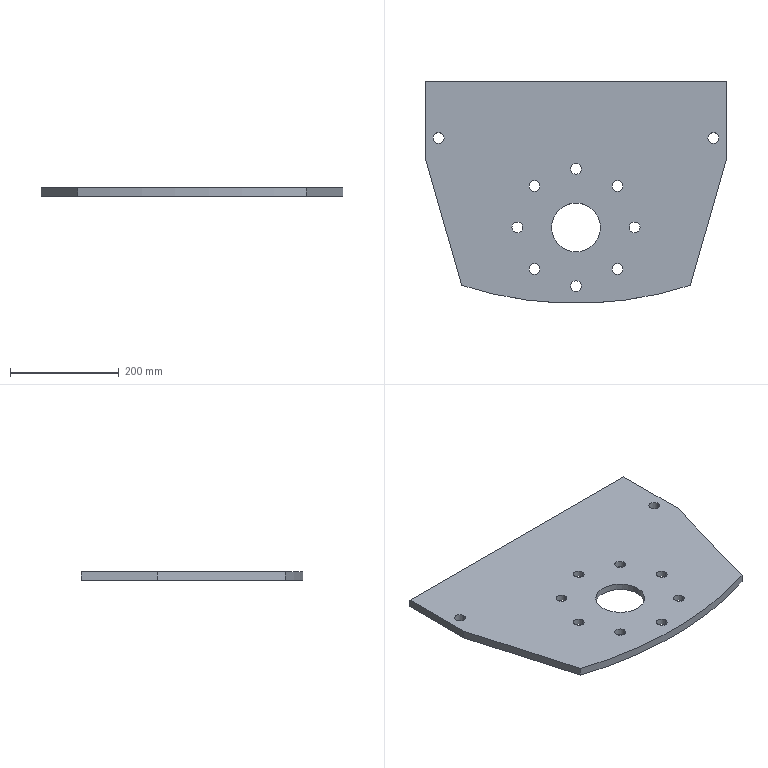Part | SolidWorks | features ICE 5, Chamfer 1, CirPattern 1, Extrusion 1, MirrorPattern 1 | 1 solid | 35 faces | box 555.5 x 409.096 x 15 mm | volume 2756721 mm3 | cylinder 25 | plane 8 | cone 2 | commonest cylinder face diameters 20 x20 90 x2 260 x2 1368 x1
STEP:
#1=CARTESIAN_POINT('',(-242.75,-105.,0.));
#2=VERTEX_POINT('',#1);
#3=CARTESIAN_POINT('',(-262.75,-105.,0.));
#4=VERTEX_POINT('',#3);
#5=CARTESIAN_POINT('',(-252.75,-105.,0.));
#6=DIRECTION('',(0.,0.,-1.));
#7=DIRECTION('',(-1.,0.,0.));
#8=AXIS2_PLACEMENT_3D('',#5,#6,#7);
#9=CIRCLE('',#8,10.);
#10=EDGE_CURVE('',#2,#4,#9,.T.);
#11=ORIENTED_EDGE('',*,*,#10,.T.);
#12=CARTESIAN_POINT('',(-262.75,-105.,15.));
#13=VERTEX_POINT('',#12);
#14=CARTESIAN_POINT('',(-262.75,-105.,0.));
#15=DIRECTION('',(0.,0.,1.));
#16=VECTOR('',#15,1000.);
#17=LINE('',#14,#16);
#18=EDGE_CURVE('',#4,#13,#17,.T.);
#19=ORIENTED_EDGE('',*,*,#18,.T.);
#20=CARTESIAN_POINT('',(-242.75,-105.,15.));
#21=VERTEX_POINT('',#20);
#22=CARTESIAN_POINT('',(-252.75,-105.,15.));
#23=DIRECTION('',(0.,0.,-1.));
#24=DIRECTION('',(-1.,0.,0.));
#25=AXIS2_PLACEMENT_3D('',#22,#23,#24);
#26=CIRCLE('',#25,10.);
#27=EDGE_CURVE('',#21,#13,#26,.T.);
#28=ORIENTED_EDGE('',*,*,#27,.F.);
#29=CARTESIAN_POINT('',(-242.75,-105.,0.));
#30=DIRECTION('',(0.,0.,1.));
#31=VECTOR('',#30,1000.);
#32=LINE('',#29,#31);
#33=EDGE_CURVE('',#2,#21,#32,.T.);
#34=ORIENTED_EDGE('',*,*,#33,.F.);
#35=EDGE_LOOP('',(#11,#19,#28,#34));
#36=FACE_OUTER_BOUND('',#35,.T.);
#37=CARTESIAN_POINT('',(-252.75,-105.,0.));
#38=DIRECTION('',(0.,0.,1.));
#39=DIRECTION('',(1.,0.,0.));
#40=AXIS2_PLACEMENT_3D('',#37,#38,#39);
#41=CYLINDRICAL_SURFACE('',#40,10.);
#42=ADVANCED_FACE('',(#36),#41,.F.);
#43=CARTESIAN_POINT('',(242.75,-105.,0.));
#44=VERTEX_POINT('',#43);
#45=CARTESIAN_POINT('',(262.75,-105.,0.));
#46=VERTEX_POINT('',#45);
#47=CARTESIAN_POINT('',(252.75,-105.,0.));
#48=DIRECTION('',(0.,0.,1.));
#49=DIRECTION('',(1.,0.,0.));
#50=AXIS2_PLACEMENT_3D('',#47,#48,#49);
#51=CIRCLE('',#50,10.);
#52=EDGE_CURVE('',#44,#46,#51,.T.);
#53=ORIENTED_EDGE('',*,*,#52,.F.);
#54=CARTESIAN_POINT('',(242.75,-105.,15.));
#55=VERTEX_POINT('',#54);
#56=CARTESIAN_POINT('',(242.75,-105.,0.));
#57=DIRECTION('',(0.,0.,1.));
#58=VECTOR('',#57,1000.);
#59=LINE('',#56,#58);
#60=EDGE_CURVE('',#44,#55,#59,.T.);
#61=ORIENTED_EDGE('',*,*,#60,.T.);
#62=CARTESIAN_POINT('',(262.75,-105.,15.));
#63=VERTEX_POINT('',#62);
#64=CARTESIAN_POINT('',(252.75,-105.,15.));
#65=DIRECTION('',(0.,0.,1.));
#66=DIRECTION('',(1.,0.,0.));
#67=AXIS2_PLACEMENT_3D('',#64,#65,#66);
#68=CIRCLE('',#67,10.);
#69=EDGE_CURVE('',#55,#63,#68,.T.);
#70=ORIENTED_EDGE('',*,*,#69,.T.);
#71=CARTESIAN_POINT('',(262.75,-105.,0.));
#72=DIRECTION('',(0.,0.,1.));
#73=VECTOR('',#72,1000.);
#74=LINE('',#71,#73);
#75=EDGE_CURVE('',#46,#63,#74,.T.);
#76=ORIENTED_EDGE('',*,*,#75,.F.);
#77=EDGE_LOOP('',(#53,#61,#70,#76));
#78=FACE_OUTER_BOUND('',#77,.T.);
#79=CARTESIAN_POINT('',(252.75,-105.,0.));
#80=DIRECTION('',(0.,0.,1.));
#81=DIRECTION('',(1.,0.,0.));
#82=AXIS2_PLACEMENT_3D('',#79,#80,#81);
#83=CYLINDRICAL_SURFACE('',#82,10.);
#84=ADVANCED_FACE('',(#78),#83,.F.);
#85=CARTESIAN_POINT('',(45.,-269.4,15.));
#86=VERTEX_POINT('',#85);
#87=CARTESIAN_POINT('',(-45.,-269.4,15.));
#88=VERTEX_POINT('',#87);
#89=CARTESIAN_POINT('',(0.,-269.4,15.));
#90=DIRECTION('',(0.,0.,-1.));
#91=DIRECTION('',(-1.,0.,0.));
#92=AXIS2_PLACEMENT_3D('',#89,#90,#91);
#93=CIRCLE('',#92,45.);
#94=EDGE_CURVE('',#86,#88,#93,.T.);
#95=ORIENTED_EDGE('',*,*,#94,.F.);
#96=CARTESIAN_POINT('',(45.,-269.4,3.));
#97=VERTEX_POINT('',#96);
#98=CARTESIAN_POINT('',(45.,-269.4,15.));
#99=DIRECTION('',(0.,0.,-1.));
#100=VECTOR('',#99,1000.);
#101=LINE('',#98,#100);
#102=EDGE_CURVE('',#86,#97,#101,.T.);
#103=ORIENTED_EDGE('',*,*,#102,.T.);
#104=CARTESIAN_POINT('',(-45.,-269.4,3.));
#105=VERTEX_POINT('',#104);
#106=CARTESIAN_POINT('',(0.,-269.4,3.));
#107=DIRECTION('',(0.,0.,-1.));
#108=DIRECTION('',(-1.,0.,0.));
#109=AXIS2_PLACEMENT_3D('',#106,#107,#108);
#110=CIRCLE('',#109,45.);
#111=EDGE_CURVE('',#97,#105,#110,.T.);
#112=ORIENTED_EDGE('',*,*,#111,.T.);
#113=CARTESIAN_POINT('',(-45.,-269.4,15.));
#114=DIRECTION('',(0.,0.,-1.));
#115=VECTOR('',#114,1000.);
#116=LINE('',#113,#115);
#117=EDGE_CURVE('',#88,#105,#116,.T.);
#118=ORIENTED_EDGE('',*,*,#117,.F.);
#119=EDGE_LOOP('',(#95,#103,#112,#118));
#120=FACE_OUTER_BOUND('',#119,.T.);
#121=CARTESIAN_POINT('',(0.,-269.4,15.));
#122=DIRECTION('',(0.,0.,-1.));
#123=DIRECTION('',(-1.,0.,0.));
#124=AXIS2_PLACEMENT_3D('',#121,#122,#123);
#125=CYLINDRICAL_SURFACE('',#124,45.);
#126=ADVANCED_FACE('',(#120),#125,.F.);
#127=CARTESIAN_POINT('',(98.,-269.4,15.));
#128=VERTEX_POINT('',#127);
#129=CARTESIAN_POINT('',(118.,-269.4,15.));
#130=VERTEX_POINT('',#129);
#131=CARTESIAN_POINT('',(108.,-269.4,15.));
#132=DIRECTION('',(0.,0.,1.));
#133=DIRECTION('',(1.,0.,0.));
#134=AXIS2_PLACEMENT_3D('',#131,#132,#133);
#135=CIRCLE('',#134,10.);
#136=EDGE_CURVE('',#128,#130,#135,.T.);
#137=ORIENTED_EDGE('',*,*,#136,.T.);
#138=CARTESIAN_POINT('',(118.,-269.4,3.));
#139=VERTEX_POINT('',#138);
#140=CARTESIAN_POINT('',(118.,-269.4,48.));
#141=DIRECTION('',(0.,0.,-1.));
#142=VECTOR('',#141,1000.);
#143=LINE('',#140,#142);
#144=EDGE_CURVE('',#130,#139,#143,.T.);
#145=ORIENTED_EDGE('',*,*,#144,.T.);
#146=CARTESIAN_POINT('',(98.,-269.4,3.));
#147=VERTEX_POINT('',#146);
#148=CARTESIAN_POINT('',(108.,-269.4,3.));
#149=DIRECTION('',(0.,0.,-1.));
#150=DIRECTION('',(-1.,0.,0.));
#151=AXIS2_PLACEMENT_3D('',#148,#149,#150);
#152=CIRCLE('',#151,10.);
#153=EDGE_CURVE('',#139,#147,#152,.T.);
#154=ORIENTED_EDGE('',*,*,#153,.T.);
#155=CARTESIAN_POINT('',(98.,-269.4,48.));
#156=DIRECTION('',(0.,0.,-1.));
#157=VECTOR('',#156,1000.);
#158=LINE('',#155,#157);
#159=EDGE_CURVE('',#128,#147,#158,.T.);
#160=ORIENTED_EDGE('',*,*,#159,.F.);
#161=EDGE_LOOP('',(#137,#145,#154,#160));
#162=FACE_OUTER_BOUND('',#161,.T.);
#163=CARTESIAN_POINT('',(108.,-269.4,48.));
#164=DIRECTION('',(0.,0.,-1.));
#165=DIRECTION('',(-1.,0.,0.));
#166=AXIS2_PLACEMENT_3D('',#163,#164,#165);
#167=CYLINDRICAL_SURFACE('',#166,10.);
#168=ADVANCED_FACE('',(#162),#167,.F.);
#169=CARTESIAN_POINT('',(66.368,-345.768,15.));
#170=VERTEX_POINT('',#169);
#171=CARTESIAN_POINT('',(86.368,-345.768,15.));
#172=VERTEX_POINT('',#171);
#173=CARTESIAN_POINT('',(76.368,-345.768,15.));
#174=DIRECTION('',(0.,0.,1.));
#175=DIRECTION('',(1.,0.,0.));
#176=AXIS2_PLACEMENT_3D('',#173,#174,#175);
#177=CIRCLE('',#176,10.);
#178=EDGE_CURVE('',#170,#172,#177,.T.);
#179=ORIENTED_EDGE('',*,*,#178,.T.);
#180=CARTESIAN_POINT('',(86.368,-345.768,3.));
#181=VERTEX_POINT('',#180);
#182=CARTESIAN_POINT('',(86.368,-345.768,48.));
#183=DIRECTION('',(0.,0.,-1.));
#184=VECTOR('',#183,1000.);
#185=LINE('',#182,#184);
#186=EDGE_CURVE('',#172,#181,#185,.T.);
#187=ORIENTED_EDGE('',*,*,#186,.T.);
#188=CARTESIAN_POINT('',(66.368,-345.768,3.));
#189=VERTEX_POINT('',#188);
#190=CARTESIAN_POINT('',(76.368,-345.768,3.));
#191=DIRECTION('',(0.,0.,-1.));
#192=DIRECTION('',(-1.,0.,0.));
#193=AXIS2_PLACEMENT_3D('',#190,#191,#192);
#194=CIRCLE('',#193,10.);
#195=EDGE_CURVE('',#181,#189,#194,.T.);
#196=ORIENTED_EDGE('',*,*,#195,.T.);
#197=CARTESIAN_POINT('',(66.368,-345.768,48.));
#198=DIRECTION('',(0.,0.,-1.));
#199=VECTOR('',#198,1000.);
#200=LINE('',#197,#199);
#201=EDGE_CURVE('',#170,#189,#200,.T.);
#202=ORIENTED_EDGE('',*,*,#201,.F.);
#203=EDGE_LOOP('',(#179,#187,#196,#202));
#204=FACE_OUTER_BOUND('',#203,.T.);
#205=CARTESIAN_POINT('',(76.368,-345.768,48.));
#206=DIRECTION('',(0.,0.,-1.));
#207=DIRECTION('',(-1.,0.,0.));
#208=AXIS2_PLACEMENT_3D('',#205,#206,#207);
#209=CYLINDRICAL_SURFACE('',#208,10.);
#210=ADVANCED_FACE('',(#204),#209,.F.);
#211=CARTESIAN_POINT('',(-10.,-377.4,15.));
#212=VERTEX_POINT('',#211);
#213=CARTESIAN_POINT('',(10.,-377.4,15.));
#214=VERTEX_POINT('',#213);
#215=CARTESIAN_POINT('',(0.,-377.4,15.));
#216=DIRECTION('',(0.,0.,1.));
#217=DIRECTION('',(1.,0.,0.));
#218=AXIS2_PLACEMENT_3D('',#215,#216,#217);
#219=CIRCLE('',#218,10.);
#220=EDGE_CURVE('',#212,#214,#219,.T.);
#221=ORIENTED_EDGE('',*,*,#220,.T.);
#222=CARTESIAN_POINT('',(10.,-377.4,3.));
#223=VERTEX_POINT('',#222);
#224=CARTESIAN_POINT('',(10.,-377.4,48.));
#225=DIRECTION('',(0.,0.,-1.));
#226=VECTOR('',#225,1000.);
#227=LINE('',#224,#226);
#228=EDGE_CURVE('',#214,#223,#227,.T.);
#229=ORIENTED_EDGE('',*,*,#228,.T.);
#230=CARTESIAN_POINT('',(-10.,-377.4,3.));
#231=VERTEX_POINT('',#230);
#232=CARTESIAN_POINT('',(0.,-377.4,3.));
#233=DIRECTION('',(0.,0.,-1.));
#234=DIRECTION('',(-1.,0.,0.));
#235=AXIS2_PLACEMENT_3D('',#232,#233,#234);
#236=CIRCLE('',#235,10.);
#237=EDGE_CURVE('',#223,#231,#236,.T.);
#238=ORIENTED_EDGE('',*,*,#237,.T.);
#239=CARTESIAN_POINT('',(-10.,-377.4,48.));
#240=DIRECTION('',(0.,0.,-1.));
#241=VECTOR('',#240,1000.);
#242=LINE('',#239,#241);
#243=EDGE_CURVE('',#212,#231,#242,.T.);
#244=ORIENTED_EDGE('',*,*,#243,.F.);
#245=EDGE_LOOP('',(#221,#229,#238,#244));
#246=FACE_OUTER_BOUND('',#245,.T.);
#247=CARTESIAN_POINT('',(0.,-377.4,48.));
#248=DIRECTION('',(0.,0.,-1.));
#249=DIRECTION('',(-1.,0.,0.));
#250=AXIS2_PLACEMENT_3D('',#247,#248,#249);
#251=CYLINDRICAL_SURFACE('',#250,10.);
#252=ADVANCED_FACE('',(#246),#251,.F.);
#253=CARTESIAN_POINT('',(-86.368,-345.768,15.));
#254=VERTEX_POINT('',#253);
#255=CARTESIAN_POINT('',(-66.368,-345.768,15.));
#256=VERTEX_POINT('',#255);
#257=CARTESIAN_POINT('',(-76.368,-345.768,15.));
#258=DIRECTION('',(0.,0.,1.));
#259=DIRECTION('',(1.,0.,0.));
#260=AXIS2_PLACEMENT_3D('',#257,#258,#259);
#261=CIRCLE('',#260,10.);
#262=EDGE_CURVE('',#254,#256,#261,.T.);
#263=ORIENTED_EDGE('',*,*,#262,.T.);
#264=CARTESIAN_POINT('',(-66.368,-345.768,3.));
#265=VERTEX_POINT('',#264);
#266=CARTESIAN_POINT('',(-66.368,-345.768,48.));
#267=DIRECTION('',(0.,0.,-1.));
#268=VECTOR('',#267,1000.);
#269=LINE('',#266,#268);
#270=EDGE_CURVE('',#256,#265,#269,.T.);
#271=ORIENTED_EDGE('',*,*,#270,.T.);
#272=CARTESIAN_POINT('',(-86.368,-345.768,3.));
#273=VERTEX_POINT('',#272);
#274=CARTESIAN_POINT('',(-76.368,-345.768,3.));
#275=DIRECTION('',(0.,0.,-1.));
#276=DIRECTION('',(-1.,0.,0.));
#277=AXIS2_PLACEMENT_3D('',#274,#275,#276);
#278=CIRCLE('',#277,10.);
#279=EDGE_CURVE('',#265,#273,#278,.T.);
#280=ORIENTED_EDGE('',*,*,#279,.T.);
#281=CARTESIAN_POINT('',(-86.368,-345.768,48.));
#282=DIRECTION('',(0.,0.,-1.));
#283=VECTOR('',#282,1000.);
#284=LINE('',#281,#283);
#285=EDGE_CURVE('',#254,#273,#284,.T.);
#286=ORIENTED_EDGE('',*,*,#285,.F.);
#287=EDGE_LOOP('',(#263,#271,#280,#286));
#288=FACE_OUTER_BOUND('',#287,.T.);
#289=CARTESIAN_POINT('',(-76.368,-345.768,48.));
#290=DIRECTION('',(0.,0.,-1.));
#291=DIRECTION('',(-1.,0.,0.));
#292=AXIS2_PLACEMENT_3D('',#289,#290,#291);
#293=CYLINDRICAL_SURFACE('',#292,10.);
#294=ADVANCED_FACE('',(#288),#293,.F.);
#295=CARTESIAN_POINT('',(-118.,-269.4,15.));
#296=VERTEX_POINT('',#295);
#297=CARTESIAN_POINT('',(-98.,-269.4,15.));
#298=VERTEX_POINT('',#297);
#299=CARTESIAN_POINT('',(-108.,-269.4,15.));
#300=DIRECTION('',(0.,0.,1.));
#301=DIRECTION('',(1.,0.,0.));
#302=AXIS2_PLACEMENT_3D('',#299,#300,#301);
#303=CIRCLE('',#302,10.);
#304=EDGE_CURVE('',#296,#298,#303,.T.);
#305=ORIENTED_EDGE('',*,*,#304,.T.);
#306=CARTESIAN_POINT('',(-98.,-269.4,3.));
#307=VERTEX_POINT('',#306);
#308=CARTESIAN_POINT('',(-98.,-269.4,48.));
#309=DIRECTION('',(0.,0.,-1.));
#310=VECTOR('',#309,1000.);
#311=LINE('',#308,#310);
#312=EDGE_CURVE('',#298,#307,#311,.T.);
#313=ORIENTED_EDGE('',*,*,#312,.T.);
#314=CARTESIAN_POINT('',(-118.,-269.4,3.));
#315=VERTEX_POINT('',#314);
#316=CARTESIAN_POINT('',(-108.,-269.4,3.));
#317=DIRECTION('',(0.,0.,-1.));
#318=DIRECTION('',(-1.,0.,0.));
#319=AXIS2_PLACEMENT_3D('',#316,#317,#318);
#320=CIRCLE('',#319,10.);
#321=EDGE_CURVE('',#307,#315,#320,.T.);
#322=ORIENTED_EDGE('',*,*,#321,.T.);
#323=CARTESIAN_POINT('',(-118.,-269.4,48.));
#324=DIRECTION('',(0.,0.,-1.));
#325=VECTOR('',#324,1000.);
#326=LINE('',#323,#325);
#327=EDGE_CURVE('',#296,#315,#326,.T.);
#328=ORIENTED_EDGE('',*,*,#327,.F.);
#329=EDGE_LOOP('',(#305,#313,#322,#328));
#330=FACE_OUTER_BOUND('',#329,.T.);
#331=CARTESIAN_POINT('',(-108.,-269.4,48.));
#332=DIRECTION('',(0.,0.,-1.));
#333=DIRECTION('',(-1.,0.,0.));
#334=AXIS2_PLACEMENT_3D('',#331,#332,#333);
#335=CYLINDRICAL_SURFACE('',#334,10.);
#336=ADVANCED_FACE('',(#330),#335,.F.);
#337=CARTESIAN_POINT('',(-86.368,-193.032,15.));
#338=VERTEX_POINT('',#337);
#339=CARTESIAN_POINT('',(-66.368,-193.032,15.));
#340=VERTEX_POINT('',#339);
#341=CARTESIAN_POINT('',(-76.368,-193.032,15.));
#342=DIRECTION('',(0.,0.,1.));
#343=DIRECTION('',(1.,0.,0.));
#344=AXIS2_PLACEMENT_3D('',#341,#342,#343);
#345=CIRCLE('',#344,10.);
#346=EDGE_CURVE('',#338,#340,#345,.T.);
#347=ORIENTED_EDGE('',*,*,#346,.T.);
#348=CARTESIAN_POINT('',(-66.368,-193.032,3.));
#349=VERTEX_POINT('',#348);
#350=CARTESIAN_POINT('',(-66.368,-193.032,48.));
#351=DIRECTION('',(0.,0.,-1.));
#352=VECTOR('',#351,1000.);
#353=LINE('',#350,#352);
#354=EDGE_CURVE('',#340,#349,#353,.T.);
#355=ORIENTED_EDGE('',*,*,#354,.T.);
#356=CARTESIAN_POINT('',(-86.368,-193.032,3.));
#357=VERTEX_POINT('',#356);
#358=CARTESIAN_POINT('',(-76.368,-193.032,3.));
#359=DIRECTION('',(0.,0.,-1.));
#360=DIRECTION('',(-1.,0.,0.));
#361=AXIS2_PLACEMENT_3D('',#358,#359,#360);
#362=CIRCLE('',#361,10.);
#363=EDGE_CURVE('',#349,#357,#362,.T.);
#364=ORIENTED_EDGE('',*,*,#363,.T.);
#365=CARTESIAN_POINT('',(-86.368,-193.032,48.));
#366=DIRECTION('',(0.,0.,-1.));
#367=VECTOR('',#366,1000.);
#368=LINE('',#365,#367);
#369=EDGE_CURVE('',#338,#357,#368,.T.);
#370=ORIENTED_EDGE('',*,*,#369,.F.);
#371=EDGE_LOOP('',(#347,#355,#364,#370));
#372=FACE_OUTER_BOUND('',#371,.T.);
#373=CARTESIAN_POINT('',(-76.368,-193.032,48.));
#374=DIRECTION('',(0.,0.,-1.));
#375=DIRECTION('',(-1.,0.,0.));
#376=AXIS2_PLACEMENT_3D('',#373,#374,#375);
#377=CYLINDRICAL_SURFACE('',#376,10.);
#378=ADVANCED_FACE('',(#372),#377,.F.);
#379=CARTESIAN_POINT('',(66.368,-193.032,15.));
#380=VERTEX_POINT('',#379);
#381=CARTESIAN_POINT('',(86.368,-193.032,15.));
#382=VERTEX_POINT('',#381);
#383=CARTESIAN_POINT('',(76.368,-193.032,15.));
#384=DIRECTION('',(0.,0.,1.));
#385=DIRECTION('',(1.,0.,0.));
#386=AXIS2_PLACEMENT_3D('',#383,#384,#385);
#387=CIRCLE('',#386,10.);
#388=EDGE_CURVE('',#380,#382,#387,.T.);
#389=ORIENTED_EDGE('',*,*,#388,.T.);
#390=CARTESIAN_POINT('',(86.368,-193.032,3.));
#391=VERTEX_POINT('',#390);
#392=CARTESIAN_POINT('',(86.368,-193.032,48.));
#393=DIRECTION('',(0.,0.,-1.));
#394=VECTOR('',#393,1000.);
#395=LINE('',#392,#394);
#396=EDGE_CURVE('',#382,#391,#395,.T.);
#397=ORIENTED_EDGE('',*,*,#396,.T.);
#398=CARTESIAN_POINT('',(66.368,-193.032,3.));
#399=VERTEX_POINT('',#398);
#400=CARTESIAN_POINT('',(76.368,-193.032,3.));
#401=DIRECTION('',(0.,0.,-1.));
#402=DIRECTION('',(-1.,0.,0.));
#403=AXIS2_PLACEMENT_3D('',#400,#401,#402);
#404=CIRCLE('',#403,10.);
#405=EDGE_CURVE('',#391,#399,#404,.T.);
#406=ORIENTED_EDGE('',*,*,#405,.T.);
#407=CARTESIAN_POINT('',(66.368,-193.032,48.));
#408=DIRECTION('',(0.,0.,-1.));
#409=VECTOR('',#408,1000.);
#410=LINE('',#407,#409);
#411=EDGE_CURVE('',#380,#399,#410,.T.);
#412=ORIENTED_EDGE('',*,*,#411,.F.);
#413=EDGE_LOOP('',(#389,#397,#406,#412));
#414=FACE_OUTER_BOUND('',#413,.T.);
#415=CARTESIAN_POINT('',(76.368,-193.032,48.));
#416=DIRECTION('',(0.,0.,-1.));
#417=DIRECTION('',(-1.,0.,0.));
#418=AXIS2_PLACEMENT_3D('',#415,#416,#417);
#419=CYLINDRICAL_SURFACE('',#418,10.);
#420=ADVANCED_FACE('',(#414),#419,.F.);
#421=CARTESIAN_POINT('',(-10.,-161.4,15.));
#422=VERTEX_POINT('',#421);
#423=CARTESIAN_POINT('',(10.,-161.4,15.));
#424=VERTEX_POINT('',#423);
#425=CARTESIAN_POINT('',(0.,-161.4,15.));
#426=DIRECTION('',(0.,0.,1.));
#427=DIRECTION('',(1.,0.,0.));
#428=AXIS2_PLACEMENT_3D('',#425,#426,#427);
#429=CIRCLE('',#428,10.);
#430=EDGE_CURVE('',#422,#424,#429,.T.);
#431=ORIENTED_EDGE('',*,*,#430,.T.);
#432=CARTESIAN_POINT('',(10.,-161.4,3.));
#433=VERTEX_POINT('',#432);
#434=CARTESIAN_POINT('',(10.,-161.4,48.));
#435=DIRECTION('',(0.,0.,-1.));
#436=VECTOR('',#435,1000.);
#437=LINE('',#434,#436);
#438=EDGE_CURVE('',#424,#433,#437,.T.);
#439=ORIENTED_EDGE('',*,*,#438,.T.);
#440=CARTESIAN_POINT('',(-10.,-161.4,3.));
#441=VERTEX_POINT('',#440);
#442=CARTESIAN_POINT('',(0.,-161.4,3.));
#443=DIRECTION('',(0.,0.,-1.));
#444=DIRECTION('',(-1.,0.,0.));
#445=AXIS2_PLACEMENT_3D('',#442,#443,#444);
#446=CIRCLE('',#445,10.);
#447=EDGE_CURVE('',#433,#441,#446,.T.);
#448=ORIENTED_EDGE('',*,*,#447,.T.);
#449=CARTESIAN_POINT('',(-10.,-161.4,48.));
#450=DIRECTION('',(0.,0.,-1.));
#451=VECTOR('',#450,1000.);
#452=LINE('',#449,#451);
#453=EDGE_CURVE('',#422,#441,#452,.T.);
#454=ORIENTED_EDGE('',*,*,#453,.F.);
#455=EDGE_LOOP('',(#431,#439,#448,#454));
#456=FACE_OUTER_BOUND('',#455,.T.);
#457=CARTESIAN_POINT('',(0.,-161.4,48.));
#458=DIRECTION('',(0.,0.,-1.));
#459=DIRECTION('',(-1.,0.,0.));
#460=AXIS2_PLACEMENT_3D('',#457,#458,#459);
#461=CYLINDRICAL_SURFACE('',#460,10.);
#462=ADVANCED_FACE('',(#456),#461,.F.);
#463=CARTESIAN_POINT('',(130.,-269.4,2.));
#464=VERTEX_POINT('',#463);
#465=CARTESIAN_POINT('',(-130.,-269.4,2.));
#466=VERTEX_POINT('',#465);
#467=CARTESIAN_POINT('',(0.,-269.4,2.));
#468=DIRECTION('',(0.,0.,-1.));
#469=DIRECTION('',(1.,0.,0.));
#470=AXIS2_PLACEMENT_3D('',#467,#468,#469);
#471=CIRCLE('',#470,130.);
#472=EDGE_CURVE('',#464,#466,#471,.T.);
#473=ORIENTED_EDGE('',*,*,#472,.F.);
#474=CARTESIAN_POINT('',(132.,-269.4,0.));
#475=VERTEX_POINT('',#474);
#476=CARTESIAN_POINT('',(130.,-269.4,2.));
#477=DIRECTION('',(0.7071,0.,-0.7071));
#478=VECTOR('',#477,1000.);
#479=LINE('',#476,#478);
#480=EDGE_CURVE('',#464,#475,#479,.T.);
#481=ORIENTED_EDGE('',*,*,#480,.T.);
#482=CARTESIAN_POINT('',(-132.,-269.4,0.));
#483=VERTEX_POINT('',#482);
#484=CARTESIAN_POINT('',(0.,-269.4,0.));
#485=DIRECTION('',(0.,0.,1.));
#486=DIRECTION('',(1.,0.,0.));
#487=AXIS2_PLACEMENT_3D('',#484,#485,#486);
#488=CIRCLE('',#487,132.);
#489=EDGE_CURVE('',#483,#475,#488,.T.);
#490=ORIENTED_EDGE('',*,*,#489,.F.);
#491=CARTESIAN_POINT('',(-130.,-269.4,2.));
#492=DIRECTION('',(-0.7071,0.,-0.7071));
#493=VECTOR('',#492,1000.);
#494=LINE('',#491,#493);
#495=EDGE_CURVE('',#466,#483,#494,.T.);
#496=ORIENTED_EDGE('',*,*,#495,.F.);
#497=EDGE_LOOP('',(#473,#481,#490,#496));
#498=FACE_OUTER_BOUND('',#497,.T.);
#499=CARTESIAN_POINT('',(0.,-269.4,2.));
#500=DIRECTION('',(0.,0.,-1.));
#501=DIRECTION('',(-1.,0.,0.));
#502=AXIS2_PLACEMENT_3D('',#499,#500,#501);
#503=CONICAL_SURFACE('',#502,130.,0.7854);
#504=ADVANCED_FACE('',(#498),#503,.F.);
#505=CARTESIAN_POINT('',(130.,-269.4,3.));
#506=VERTEX_POINT('',#505);
#507=CARTESIAN_POINT('',(-130.,-269.4,3.));
#508=VERTEX_POINT('',#507);
#509=CARTESIAN_POINT('',(0.,-269.4,3.));
#510=DIRECTION('',(0.,0.,-1.));
#511=DIRECTION('',(-1.,0.,0.));
#512=AXIS2_PLACEMENT_3D('',#509,#510,#511);
#513=CIRCLE('',#512,130.);
#514=EDGE_CURVE('',#506,#508,#513,.T.);
#515=ORIENTED_EDGE('',*,*,#514,.F.);
#516=CARTESIAN_POINT('',(130.,-269.4,3.));
#517=DIRECTION('',(0.,0.,-1.));
#518=VECTOR('',#517,1000.);
#519=LINE('',#516,#518);
#520=EDGE_CURVE('',#506,#464,#519,.T.);
#521=ORIENTED_EDGE('',*,*,#520,.T.);
#522=ORIENTED_EDGE('',*,*,#472,.T.);
#523=CARTESIAN_POINT('',(-130.,-269.4,3.));
#524=DIRECTION('',(0.,0.,-1.));
#525=VECTOR('',#524,1000.);
#526=LINE('',#523,#525);
#527=EDGE_CURVE('',#508,#466,#526,.T.);
#528=ORIENTED_EDGE('',*,*,#527,.F.);
#529=EDGE_LOOP('',(#515,#521,#522,#528));
#530=FACE_OUTER_BOUND('',#529,.T.);
#531=CARTESIAN_POINT('',(0.,-269.4,3.));
#532=DIRECTION('',(0.,0.,-1.));
#533=DIRECTION('',(-1.,0.,0.));
#534=AXIS2_PLACEMENT_3D('',#531,#532,#533);
#535=CYLINDRICAL_SURFACE('',#534,130.);
#536=ADVANCED_FACE('',(#530),#535,.F.);
#537=CARTESIAN_POINT('',(277.75,-140.,15.));
#538=VERTEX_POINT('',#537);
#539=CARTESIAN_POINT('',(210.161,-376.005,15.));
#540=VERTEX_POINT('',#539);
#541=CARTESIAN_POINT('',(293.751,-84.127,15.));
#542=DIRECTION('',(-0.2753,-0.9614,0.));
#543=VECTOR('',#542,1000.);
#544=LINE('',#541,#543);
#545=EDGE_CURVE('',#538,#540,#544,.T.);
#546=ORIENTED_EDGE('',*,*,#545,.T.);
#547=CARTESIAN_POINT('',(210.161,-376.005,0.));
#548=VERTEX_POINT('',#547);
#549=CARTESIAN_POINT('',(210.161,-376.005,-35.));
#550=DIRECTION('',(0.,0.,-1.));
#551=VECTOR('',#550,1000.);
#552=LINE('',#549,#551);
#553=EDGE_CURVE('',#540,#548,#552,.T.);
#554=ORIENTED_EDGE('',*,*,#553,.T.);
#555=CARTESIAN_POINT('',(277.75,-140.,0.));
#556=VERTEX_POINT('',#555);
#557=CARTESIAN_POINT('',(293.751,-84.127,0.));
#558=DIRECTION('',(-0.2753,-0.9614,0.));
#559=VECTOR('',#558,1000.);
#560=LINE('',#557,#559);
#561=EDGE_CURVE('',#556,#548,#560,.T.);
#562=ORIENTED_EDGE('',*,*,#561,.F.);
#563=CARTESIAN_POINT('',(277.75,-140.,15.));
#564=DIRECTION('',(0.,0.,-1.));
#565=VECTOR('',#564,1000.);
#566=LINE('',#563,#565);
#567=EDGE_CURVE('',#538,#556,#566,.T.);
#568=ORIENTED_EDGE('',*,*,#567,.F.);
#569=EDGE_LOOP('',(#546,#554,#562,#568));
#570=FACE_OUTER_BOUND('',#569,.T.);
#571=CARTESIAN_POINT('',(293.751,-84.127,15.));
#572=DIRECTION('',(0.9614,-0.2753,0.));
#573=DIRECTION('',(0.2753,0.9614,0.));
#574=AXIS2_PLACEMENT_3D('',#571,#572,#573);
#575=PLANE('',#574);
#576=ADVANCED_FACE('',(#570),#575,.T.);
#577=CARTESIAN_POINT('',(-210.161,-376.005,15.));
#578=VERTEX_POINT('',#577);
#579=CARTESIAN_POINT('',(-210.161,-376.005,0.));
#580=VERTEX_POINT('',#579);
#581=CARTESIAN_POINT('',(-210.161,-376.005,-35.));
#582=DIRECTION('',(0.,0.,-1.));
#583=VECTOR('',#582,1000.);
#584=LINE('',#581,#583);
#585=EDGE_CURVE('',#578,#580,#584,.T.);
#586=ORIENTED_EDGE('',*,*,#585,.F.);
#587=CARTESIAN_POINT('',(-277.75,-140.,15.));
#588=VERTEX_POINT('',#587);
#589=CARTESIAN_POINT('',(-293.751,-84.127,15.));
#590=DIRECTION('',(0.2753,-0.9614,0.));
#591=VECTOR('',#590,1000.);
#592=LINE('',#589,#591);
#593=EDGE_CURVE('',#588,#578,#592,.T.);
#594=ORIENTED_EDGE('',*,*,#593,.F.);
#595=CARTESIAN_POINT('',(-277.75,-140.,0.));
#596=VERTEX_POINT('',#595);
#597=CARTESIAN_POINT('',(-277.75,-140.,15.));
#598=DIRECTION('',(0.,0.,-1.));
#599=VECTOR('',#598,1000.);
#600=LINE('',#597,#599);
#601=EDGE_CURVE('',#588,#596,#600,.T.);
#602=ORIENTED_EDGE('',*,*,#601,.T.);
#603=CARTESIAN_POINT('',(-293.751,-84.127,0.));
#604=DIRECTION('',(0.2753,-0.9614,0.));
#605=VECTOR('',#604,1000.);
#606=LINE('',#603,#605);
#607=EDGE_CURVE('',#596,#580,#606,.T.);
#608=ORIENTED_EDGE('',*,*,#607,.T.);
#609=EDGE_LOOP('',(#586,#594,#602,#608));
#610=FACE_OUTER_BOUND('',#609,.T.);
#611=CARTESIAN_POINT('',(-293.751,-84.127,15.));
#612=DIRECTION('',(0.9614,0.2753,0.));
#613=DIRECTION('',(-0.2753,0.9614,0.));
#614=AXIS2_PLACEMENT_3D('',#611,#612,#613);
#615=PLANE('',#614);
#616=ADVANCED_FACE('',(#610),#615,.F.);
#617=ORIENTED_EDGE('',*,*,#27,.T.);
#618=CARTESIAN_POINT('',(-252.75,-105.,15.));
#619=DIRECTION('',(0.,0.,-1.));
#620=DIRECTION('',(-1.,0.,0.));
#621=AXIS2_PLACEMENT_3D('',#618,#619,#620);
#622=CIRCLE('',#621,10.);
#623=EDGE_CURVE('',#13,#21,#622,.T.);
#624=ORIENTED_EDGE('',*,*,#623,.T.);
#625=EDGE_LOOP('',(#617,#624));
#626=FACE_BOUND('',#625,.T.);
#627=CARTESIAN_POINT('',(252.75,-105.,15.));
#628=DIRECTION('',(0.,0.,1.));
#629=DIRECTION('',(1.,0.,0.));
#630=AXIS2_PLACEMENT_3D('',#627,#628,#629);
#631=CIRCLE('',#630,10.);
#632=EDGE_CURVE('',#63,#55,#631,.T.);
#633=ORIENTED_EDGE('',*,*,#632,.F.);
#634=ORIENTED_EDGE('',*,*,#69,.F.);
#635=EDGE_LOOP('',(#633,#634));
#636=FACE_BOUND('',#635,.T.);
#637=CARTESIAN_POINT('',(0.,-269.4,15.));
#638=DIRECTION('',(0.,0.,-1.));
#639=DIRECTION('',(-1.,0.,0.));
#640=AXIS2_PLACEMENT_3D('',#637,#638,#639);
#641=CIRCLE('',#640,45.);
#642=EDGE_CURVE('',#88,#86,#641,.T.);
#643=ORIENTED_EDGE('',*,*,#642,.T.);
#644=ORIENTED_EDGE('',*,*,#94,.T.);
#645=EDGE_LOOP('',(#643,#644));
#646=FACE_BOUND('',#645,.T.);
#647=ORIENTED_EDGE('',*,*,#136,.F.);
#648=CARTESIAN_POINT('',(108.,-269.4,15.));
#649=DIRECTION('',(0.,0.,1.));
#650=DIRECTION('',(1.,0.,0.));
#651=AXIS2_PLACEMENT_3D('',#648,#649,#650);
#652=CIRCLE('',#651,10.);
#653=EDGE_CURVE('',#130,#128,#652,.T.);
#654=ORIENTED_EDGE('',*,*,#653,.F.);
#655=EDGE_LOOP('',(#647,#654));
#656=FACE_BOUND('',#655,.T.);
#657=ORIENTED_EDGE('',*,*,#178,.F.);
#658=CARTESIAN_POINT('',(76.368,-345.768,15.));
#659=DIRECTION('',(0.,0.,1.));
#660=DIRECTION('',(1.,0.,0.));
#661=AXIS2_PLACEMENT_3D('',#658,#659,#660);
#662=CIRCLE('',#661,10.);
#663=EDGE_CURVE('',#172,#170,#662,.T.);
#664=ORIENTED_EDGE('',*,*,#663,.F.);
#665=EDGE_LOOP('',(#657,#664));
#666=FACE_BOUND('',#665,.T.);
#667=ORIENTED_EDGE('',*,*,#220,.F.);
#668=CARTESIAN_POINT('',(0.,-377.4,15.));
#669=DIRECTION('',(0.,0.,1.));
#670=DIRECTION('',(1.,0.,0.));
#671=AXIS2_PLACEMENT_3D('',#668,#669,#670);
#672=CIRCLE('',#671,10.);
#673=EDGE_CURVE('',#214,#212,#672,.T.);
#674=ORIENTED_EDGE('',*,*,#673,.F.);
#675=EDGE_LOOP('',(#667,#674));
#676=FACE_BOUND('',#675,.T.);
#677=ORIENTED_EDGE('',*,*,#262,.F.);
#678=CARTESIAN_POINT('',(-76.368,-345.768,15.));
#679=DIRECTION('',(0.,0.,1.));
#680=DIRECTION('',(1.,0.,0.));
#681=AXIS2_PLACEMENT_3D('',#678,#679,#680);
#682=CIRCLE('',#681,10.);
#683=EDGE_CURVE('',#256,#254,#682,.T.);
#684=ORIENTED_EDGE('',*,*,#683,.F.);
#685=EDGE_LOOP('',(#677,#684));
#686=FACE_BOUND('',#685,.T.);
#687=ORIENTED_EDGE('',*,*,#304,.F.);
#688=CARTESIAN_POINT('',(-108.,-269.4,15.));
#689=DIRECTION('',(0.,0.,1.));
#690=DIRECTION('',(1.,0.,0.));
#691=AXIS2_PLACEMENT_3D('',#688,#689,#690);
#692=CIRCLE('',#691,10.);
#693=EDGE_CURVE('',#298,#296,#692,.T.);
#694=ORIENTED_EDGE('',*,*,#693,.F.);
#695=EDGE_LOOP('',(#687,#694));
#696=FACE_BOUND('',#695,.T.);
#697=ORIENTED_EDGE('',*,*,#346,.F.);
#698=CARTESIAN_POINT('',(-76.368,-193.032,15.));
#699=DIRECTION('',(0.,0.,1.));
#700=DIRECTION('',(1.,0.,0.));
#701=AXIS2_PLACEMENT_3D('',#698,#699,#700);
#702=CIRCLE('',#701,10.);
#703=EDGE_CURVE('',#340,#338,#702,.T.);
#704=ORIENTED_EDGE('',*,*,#703,.F.);
#705=EDGE_LOOP('',(#697,#704));
#706=FACE_BOUND('',#705,.T.);
#707=ORIENTED_EDGE('',*,*,#388,.F.);
#708=CARTESIAN_POINT('',(76.368,-193.032,15.));
#709=DIRECTION('',(0.,0.,1.));
#710=DIRECTION('',(1.,0.,0.));
#711=AXIS2_PLACEMENT_3D('',#708,#709,#710);
#712=CIRCLE('',#711,10.);
#713=EDGE_CURVE('',#382,#380,#712,.T.);
#714=ORIENTED_EDGE('',*,*,#713,.F.);
#715=EDGE_LOOP('',(#707,#714));
#716=FACE_BOUND('',#715,.T.);
#717=ORIENTED_EDGE('',*,*,#430,.F.);
#718=CARTESIAN_POINT('',(0.,-161.4,15.));
#719=DIRECTION('',(0.,0.,1.));
#720=DIRECTION('',(1.,0.,0.));
#721=AXIS2_PLACEMENT_3D('',#718,#719,#720);
#722=CIRCLE('',#721,10.);
#723=EDGE_CURVE('',#424,#422,#722,.T.);
#724=ORIENTED_EDGE('',*,*,#723,.F.);
#725=EDGE_LOOP('',(#717,#724));
#726=FACE_BOUND('',#725,.T.);
#727=ORIENTED_EDGE('',*,*,#593,.T.);
#728=CARTESIAN_POINT('',(0.,274.819,15.));
#729=DIRECTION('',(0.,0.,1.));
#730=DIRECTION('',(1.,0.,0.));
#731=AXIS2_PLACEMENT_3D('',#728,#729,#730);
#732=CIRCLE('',#731,683.915);
#733=EDGE_CURVE('',#578,#540,#732,.T.);
#734=ORIENTED_EDGE('',*,*,#733,.T.);
#735=ORIENTED_EDGE('',*,*,#545,.F.);
#736=CARTESIAN_POINT('',(277.75,0.,15.));
#737=VERTEX_POINT('',#736);
#738=CARTESIAN_POINT('',(277.75,0.,15.));
#739=DIRECTION('',(0.,-1.,0.));
#740=VECTOR('',#739,1000.);
#741=LINE('',#738,#740);
#742=EDGE_CURVE('',#737,#538,#741,.T.);
#743=ORIENTED_EDGE('',*,*,#742,.F.);
#744=CARTESIAN_POINT('',(-277.75,0.,15.));
#745=VERTEX_POINT('',#744);
#746=CARTESIAN_POINT('',(0.,0.,15.));
#747=DIRECTION('',(-1.,0.,0.));
#748=VECTOR('',#747,1000.);
#749=LINE('',#746,#748);
#750=EDGE_CURVE('',#737,#745,#749,.T.);
#751=ORIENTED_EDGE('',*,*,#750,.T.);
#752=CARTESIAN_POINT('',(-277.75,0.,15.));
#753=DIRECTION('',(0.,-1.,0.));
#754=VECTOR('',#753,1000.);
#755=LINE('',#752,#754);
#756=EDGE_CURVE('',#745,#588,#755,.T.);
#757=ORIENTED_EDGE('',*,*,#756,.T.);
#758=EDGE_LOOP('',(#727,#734,#735,#743,#751,#757));
#759=FACE_OUTER_BOUND('',#758,.T.);
#760=CARTESIAN_POINT('',(0.,0.,15.));
#761=DIRECTION('',(0.,0.,1.));
#762=DIRECTION('',(1.,0.,0.));
#763=AXIS2_PLACEMENT_3D('',#760,#761,#762);
#764=PLANE('',#763);
#765=ADVANCED_FACE('',(#626,#636,#646,#656,#666,#676,#686,#696,#706,#716,#726,#759),#764,.T.);
#766=ORIENTED_EDGE('',*,*,#10,.F.);
#767=CARTESIAN_POINT('',(-252.75,-105.,0.));
#768=DIRECTION('',(0.,0.,-1.));
#769=DIRECTION('',(-1.,0.,0.));
#770=AXIS2_PLACEMENT_3D('',#767,#768,#769);
#771=CIRCLE('',#770,10.);
#772=EDGE_CURVE('',#4,#2,#771,.T.);
#773=ORIENTED_EDGE('',*,*,#772,.F.);
#774=EDGE_LOOP('',(#766,#773));
#775=FACE_BOUND('',#774,.T.);
#776=ORIENTED_EDGE('',*,*,#489,.T.);
#777=CARTESIAN_POINT('',(0.,-269.4,0.));
#778=DIRECTION('',(0.,0.,1.));
#779=DIRECTION('',(1.,0.,0.));
#780=AXIS2_PLACEMENT_3D('',#777,#778,#779);
#781=CIRCLE('',#780,132.);
#782=EDGE_CURVE('',#475,#483,#781,.T.);
#783=ORIENTED_EDGE('',*,*,#782,.T.);
#784=EDGE_LOOP('',(#776,#783));
#785=FACE_BOUND('',#784,.T.);
#786=CARTESIAN_POINT('',(252.75,-105.,0.));
#787=DIRECTION('',(0.,0.,1.));
#788=DIRECTION('',(1.,0.,0.));
#789=AXIS2_PLACEMENT_3D('',#786,#787,#788);
#790=CIRCLE('',#789,10.);
#791=EDGE_CURVE('',#46,#44,#790,.T.);
#792=ORIENTED_EDGE('',*,*,#791,.T.);
#793=ORIENTED_EDGE('',*,*,#52,.T.);
#794=EDGE_LOOP('',(#792,#793));
#795=FACE_BOUND('',#794,.T.);
#796=CARTESIAN_POINT('',(0.,274.819,0.));
#797=DIRECTION('',(0.,0.,1.));
#798=DIRECTION('',(1.,0.,0.));
#799=AXIS2_PLACEMENT_3D('',#796,#797,#798);
#800=CIRCLE('',#799,683.915);
#801=EDGE_CURVE('',#580,#548,#800,.T.);
#802=ORIENTED_EDGE('',*,*,#801,.F.);
#803=ORIENTED_EDGE('',*,*,#607,.F.);
#804=CARTESIAN_POINT('',(-277.75,0.,0.));
#805=VERTEX_POINT('',#804);
#806=CARTESIAN_POINT('',(-277.75,0.,0.));
#807=DIRECTION('',(0.,-1.,0.));
#808=VECTOR('',#807,1000.);
#809=LINE('',#806,#808);
#810=EDGE_CURVE('',#805,#596,#809,.T.);
#811=ORIENTED_EDGE('',*,*,#810,.F.);
#812=CARTESIAN_POINT('',(277.75,0.,0.));
#813=VERTEX_POINT('',#812);
#814=CARTESIAN_POINT('',(0.,0.,0.));
#815=DIRECTION('',(-1.,0.,0.));
#816=VECTOR('',#815,1000.);
#817=LINE('',#814,#816);
#818=EDGE_CURVE('',#813,#805,#817,.T.);
#819=ORIENTED_EDGE('',*,*,#818,.F.);
#820=CARTESIAN_POINT('',(277.75,0.,0.));
#821=DIRECTION('',(0.,-1.,0.));
#822=VECTOR('',#821,1000.);
#823=LINE('',#820,#822);
#824=EDGE_CURVE('',#813,#556,#823,.T.);
#825=ORIENTED_EDGE('',*,*,#824,.T.);
#826=ORIENTED_EDGE('',*,*,#561,.T.);
#827=EDGE_LOOP('',(#802,#803,#811,#819,#825,#826));
#828=FACE_OUTER_BOUND('',#827,.T.);
#829=CARTESIAN_POINT('',(0.,0.,0.));
#830=DIRECTION('',(0.,0.,1.));
#831=DIRECTION('',(1.,0.,0.));
#832=AXIS2_PLACEMENT_3D('',#829,#830,#831);
#833=PLANE('',#832);
#834=ADVANCED_FACE('',(#775,#785,#795,#828),#833,.F.);
#835=ORIENTED_EDGE('',*,*,#824,.F.);
#836=CARTESIAN_POINT('',(277.75,0.,15.));
#837=DIRECTION('',(0.,0.,-1.));
#838=VECTOR('',#837,1000.);
#839=LINE('',#836,#838);
#840=EDGE_CURVE('',#737,#813,#839,.T.);
#841=ORIENTED_EDGE('',*,*,#840,.F.);
#842=ORIENTED_EDGE('',*,*,#742,.T.);
#843=ORIENTED_EDGE('',*,*,#567,.T.);
#844=EDGE_LOOP('',(#835,#841,#842,#843));
#845=FACE_OUTER_BOUND('',#844,.T.);
#846=CARTESIAN_POINT('',(277.75,0.,15.));
#847=DIRECTION('',(1.,0.,0.));
#848=DIRECTION('',(0.,0.,-1.));
#849=AXIS2_PLACEMENT_3D('',#846,#847,#848);
#850=PLANE('',#849);
#851=ADVANCED_FACE('',(#845),#850,.T.);
#852=ORIENTED_EDGE('',*,*,#818,.T.);
#853=CARTESIAN_POINT('',(-277.75,0.,15.));
#854=DIRECTION('',(0.,0.,-1.));
#855=VECTOR('',#854,1000.);
#856=LINE('',#853,#855);
#857=EDGE_CURVE('',#745,#805,#856,.T.);
#858=ORIENTED_EDGE('',*,*,#857,.F.);
#859=ORIENTED_EDGE('',*,*,#750,.F.);
#860=ORIENTED_EDGE('',*,*,#840,.T.);
#861=EDGE_LOOP('',(#852,#858,#859,#860));
#862=FACE_OUTER_BOUND('',#861,.T.);
#863=CARTESIAN_POINT('',(0.,0.,15.));
#864=DIRECTION('',(0.,-1.,0.));
#865=DIRECTION('',(1.,0.,0.));
#866=AXIS2_PLACEMENT_3D('',#863,#864,#865);
#867=PLANE('',#866);
#868=ADVANCED_FACE('',(#862),#867,.F.);
#869=ORIENTED_EDGE('',*,*,#810,.T.);
#870=ORIENTED_EDGE('',*,*,#601,.F.);
#871=ORIENTED_EDGE('',*,*,#756,.F.);
#872=ORIENTED_EDGE('',*,*,#857,.T.);
#873=EDGE_LOOP('',(#869,#870,#871,#872));
#874=FACE_OUTER_BOUND('',#873,.T.);
#875=CARTESIAN_POINT('',(-277.75,0.,15.));
#876=DIRECTION('',(1.,0.,0.));
#877=DIRECTION('',(0.,0.,-1.));
#878=AXIS2_PLACEMENT_3D('',#875,#876,#877);
#879=PLANE('',#878);
#880=ADVANCED_FACE('',(#874),#879,.F.);
#881=ORIENTED_EDGE('',*,*,#520,.F.);
#882=CARTESIAN_POINT('',(0.,-269.4,3.));
#883=DIRECTION('',(0.,0.,-1.));
#884=DIRECTION('',(-1.,0.,0.));
#885=AXIS2_PLACEMENT_3D('',#882,#883,#884);
#886=CIRCLE('',#885,130.);
#887=EDGE_CURVE('',#508,#506,#886,.T.);
#888=ORIENTED_EDGE('',*,*,#887,.F.);
#889=ORIENTED_EDGE('',*,*,#527,.T.);
#890=CARTESIAN_POINT('',(0.,-269.4,2.));
#891=DIRECTION('',(0.,0.,-1.));
#892=DIRECTION('',(1.,0.,0.));
#893=AXIS2_PLACEMENT_3D('',#890,#891,#892);
#894=CIRCLE('',#893,130.);
#895=EDGE_CURVE('',#466,#464,#894,.T.);
#896=ORIENTED_EDGE('',*,*,#895,.T.);
#897=EDGE_LOOP('',(#881,#888,#889,#896));
#898=FACE_OUTER_BOUND('',#897,.T.);
#899=CARTESIAN_POINT('',(0.,-269.4,3.));
#900=DIRECTION('',(0.,0.,-1.));
#901=DIRECTION('',(-1.,0.,0.));
#902=AXIS2_PLACEMENT_3D('',#899,#900,#901);
#903=CYLINDRICAL_SURFACE('',#902,130.);
#904=ADVANCED_FACE('',(#898),#903,.F.);
#905=CARTESIAN_POINT('',(0.,-269.4,3.));
#906=DIRECTION('',(0.,0.,-1.));
#907=DIRECTION('',(-1.,0.,0.));
#908=AXIS2_PLACEMENT_3D('',#905,#906,#907);
#909=CIRCLE('',#908,45.);
#910=EDGE_CURVE('',#105,#97,#909,.T.);
#911=ORIENTED_EDGE('',*,*,#910,.F.);
#912=ORIENTED_EDGE('',*,*,#111,.F.);
#913=EDGE_LOOP('',(#911,#912));
#914=FACE_BOUND('',#913,.T.);
#915=CARTESIAN_POINT('',(108.,-269.4,3.));
#916=DIRECTION('',(0.,0.,-1.));
#917=DIRECTION('',(-1.,0.,0.));
#918=AXIS2_PLACEMENT_3D('',#915,#916,#917);
#919=CIRCLE('',#918,10.);
#920=EDGE_CURVE('',#147,#139,#919,.T.);
#921=ORIENTED_EDGE('',*,*,#920,.F.);
#922=ORIENTED_EDGE('',*,*,#153,.F.);
#923=EDGE_LOOP('',(#921,#922));
#924=FACE_BOUND('',#923,.T.);
#925=CARTESIAN_POINT('',(76.368,-345.768,3.));
#926=DIRECTION('',(0.,0.,-1.));
#927=DIRECTION('',(-1.,0.,0.));
#928=AXIS2_PLACEMENT_3D('',#925,#926,#927);
#929=CIRCLE('',#928,10.);
#930=EDGE_CURVE('',#189,#181,#929,.T.);
#931=ORIENTED_EDGE('',*,*,#930,.F.);
#932=ORIENTED_EDGE('',*,*,#195,.F.);
#933=EDGE_LOOP('',(#931,#932));
#934=FACE_BOUND('',#933,.T.);
#935=CARTESIAN_POINT('',(0.,-377.4,3.));
#936=DIRECTION('',(0.,0.,-1.));
#937=DIRECTION('',(-1.,0.,0.));
#938=AXIS2_PLACEMENT_3D('',#935,#936,#937);
#939=CIRCLE('',#938,10.);
#940=EDGE_CURVE('',#231,#223,#939,.T.);
#941=ORIENTED_EDGE('',*,*,#940,.F.);
#942=ORIENTED_EDGE('',*,*,#237,.F.);
#943=EDGE_LOOP('',(#941,#942));
#944=FACE_BOUND('',#943,.T.);
#945=CARTESIAN_POINT('',(-76.368,-345.768,3.));
#946=DIRECTION('',(0.,0.,-1.));
#947=DIRECTION('',(-1.,0.,0.));
#948=AXIS2_PLACEMENT_3D('',#945,#946,#947);
#949=CIRCLE('',#948,10.);
#950=EDGE_CURVE('',#273,#265,#949,.T.);
#951=ORIENTED_EDGE('',*,*,#950,.F.);
#952=ORIENTED_EDGE('',*,*,#279,.F.);
#953=EDGE_LOOP('',(#951,#952));
#954=FACE_BOUND('',#953,.T.);
#955=CARTESIAN_POINT('',(-108.,-269.4,3.));
#956=DIRECTION('',(0.,0.,-1.));
#957=DIRECTION('',(-1.,0.,0.));
#958=AXIS2_PLACEMENT_3D('',#955,#956,#957);
#959=CIRCLE('',#958,10.);
#960=EDGE_CURVE('',#315,#307,#959,.T.);
#961=ORIENTED_EDGE('',*,*,#960,.F.);
#962=ORIENTED_EDGE('',*,*,#321,.F.);
#963=EDGE_LOOP('',(#961,#962));
#964=FACE_BOUND('',#963,.T.);
#965=CARTESIAN_POINT('',(-76.368,-193.032,3.));
#966=DIRECTION('',(0.,0.,-1.));
#967=DIRECTION('',(-1.,0.,0.));
#968=AXIS2_PLACEMENT_3D('',#965,#966,#967);
#969=CIRCLE('',#968,10.);
#970=EDGE_CURVE('',#357,#349,#969,.T.);
#971=ORIENTED_EDGE('',*,*,#970,.F.);
#972=ORIENTED_EDGE('',*,*,#363,.F.);
#973=EDGE_LOOP('',(#971,#972));
#974=FACE_BOUND('',#973,.T.);
#975=CARTESIAN_POINT('',(76.368,-193.032,3.));
#976=DIRECTION('',(0.,0.,-1.));
#977=DIRECTION('',(-1.,0.,0.));
#978=AXIS2_PLACEMENT_3D('',#975,#976,#977);
#979=CIRCLE('',#978,10.);
#980=EDGE_CURVE('',#399,#391,#979,.T.);
#981=ORIENTED_EDGE('',*,*,#980,.F.);
#982=ORIENTED_EDGE('',*,*,#405,.F.);
#983=EDGE_LOOP('',(#981,#982));
#984=FACE_BOUND('',#983,.T.);
#985=CARTESIAN_POINT('',(0.,-161.4,3.));
#986=DIRECTION('',(0.,0.,-1.));
#987=DIRECTION('',(-1.,0.,0.));
#988=AXIS2_PLACEMENT_3D('',#985,#986,#987);
#989=CIRCLE('',#988,10.);
#990=EDGE_CURVE('',#441,#433,#989,.T.);
#991=ORIENTED_EDGE('',*,*,#990,.F.);
#992=ORIENTED_EDGE('',*,*,#447,.F.);
#993=EDGE_LOOP('',(#991,#992));
#994=FACE_BOUND('',#993,.T.);
#995=ORIENTED_EDGE('',*,*,#887,.T.);
#996=ORIENTED_EDGE('',*,*,#514,.T.);
#997=EDGE_LOOP('',(#995,#996));
#998=FACE_OUTER_BOUND('',#997,.T.);
#999=CARTESIAN_POINT('',(0.,0.,3.));
#1000=DIRECTION('',(0.,0.,-1.));
#1001=DIRECTION('',(-1.,0.,0.));
#1002=AXIS2_PLACEMENT_3D('',#999,#1000,#1001);
#1003=PLANE('',#1002);
#1004=ADVANCED_FACE('',(#914,#924,#934,#944,#954,#964,#974,#984,#994,#998),#1003,.T.);
#1005=ORIENTED_EDGE('',*,*,#480,.F.);
#1006=ORIENTED_EDGE('',*,*,#895,.F.);
#1007=ORIENTED_EDGE('',*,*,#495,.T.);
#1008=ORIENTED_EDGE('',*,*,#782,.F.);
#1009=EDGE_LOOP('',(#1005,#1006,#1007,#1008));
#1010=FACE_OUTER_BOUND('',#1009,.T.);
#1011=CARTESIAN_POINT('',(0.,-269.4,2.));
#1012=DIRECTION('',(0.,0.,-1.));
#1013=DIRECTION('',(-1.,0.,0.));
#1014=AXIS2_PLACEMENT_3D('',#1011,#1012,#1013);
#1015=CONICAL_SURFACE('',#1014,130.,0.7854);
#1016=ADVANCED_FACE('',(#1010),#1015,.F.);
#1017=ORIENTED_EDGE('',*,*,#438,.F.);
#1018=ORIENTED_EDGE('',*,*,#723,.T.);
#1019=ORIENTED_EDGE('',*,*,#453,.T.);
#1020=ORIENTED_EDGE('',*,*,#990,.T.);
#1021=EDGE_LOOP('',(#1017,#1018,#1019,#1020));
#1022=FACE_OUTER_BOUND('',#1021,.T.);
#1023=CARTESIAN_POINT('',(0.,-161.4,48.));
#1024=DIRECTION('',(0.,0.,-1.));
#1025=DIRECTION('',(-1.,0.,0.));
#1026=AXIS2_PLACEMENT_3D('',#1023,#1024,#1025);
#1027=CYLINDRICAL_SURFACE('',#1026,10.);
#1028=ADVANCED_FACE('',(#1022),#1027,.F.);
#1029=ORIENTED_EDGE('',*,*,#396,.F.);
#1030=ORIENTED_EDGE('',*,*,#713,.T.);
#1031=ORIENTED_EDGE('',*,*,#411,.T.);
#1032=ORIENTED_EDGE('',*,*,#980,.T.);
#1033=EDGE_LOOP('',(#1029,#1030,#1031,#1032));
#1034=FACE_OUTER_BOUND('',#1033,.T.);
#1035=CARTESIAN_POINT('',(76.368,-193.032,48.));
#1036=DIRECTION('',(0.,0.,-1.));
#1037=DIRECTION('',(-1.,0.,0.));
#1038=AXIS2_PLACEMENT_3D('',#1035,#1036,#1037);
#1039=CYLINDRICAL_SURFACE('',#1038,10.);
#1040=ADVANCED_FACE('',(#1034),#1039,.F.);
#1041=ORIENTED_EDGE('',*,*,#354,.F.);
#1042=ORIENTED_EDGE('',*,*,#703,.T.);
#1043=ORIENTED_EDGE('',*,*,#369,.T.);
#1044=ORIENTED_EDGE('',*,*,#970,.T.);
#1045=EDGE_LOOP('',(#1041,#1042,#1043,#1044));
#1046=FACE_OUTER_BOUND('',#1045,.T.);
#1047=CARTESIAN_POINT('',(-76.368,-193.032,48.));
#1048=DIRECTION('',(0.,0.,-1.));
#1049=DIRECTION('',(-1.,0.,0.));
#1050=AXIS2_PLACEMENT_3D('',#1047,#1048,#1049);
#1051=CYLINDRICAL_SURFACE('',#1050,10.);
#1052=ADVANCED_FACE('',(#1046),#1051,.F.);
#1053=ORIENTED_EDGE('',*,*,#312,.F.);
#1054=ORIENTED_EDGE('',*,*,#693,.T.);
#1055=ORIENTED_EDGE('',*,*,#327,.T.);
#1056=ORIENTED_EDGE('',*,*,#960,.T.);
#1057=EDGE_LOOP('',(#1053,#1054,#1055,#1056));
#1058=FACE_OUTER_BOUND('',#1057,.T.);
#1059=CARTESIAN_POINT('',(-108.,-269.4,48.));
#1060=DIRECTION('',(0.,0.,-1.));
#1061=DIRECTION('',(-1.,0.,0.));
#1062=AXIS2_PLACEMENT_3D('',#1059,#1060,#1061);
#1063=CYLINDRICAL_SURFACE('',#1062,10.);
#1064=ADVANCED_FACE('',(#1058),#1063,.F.);
#1065=ORIENTED_EDGE('',*,*,#270,.F.);
#1066=ORIENTED_EDGE('',*,*,#683,.T.);
#1067=ORIENTED_EDGE('',*,*,#285,.T.);
#1068=ORIENTED_EDGE('',*,*,#950,.T.);
#1069=EDGE_LOOP('',(#1065,#1066,#1067,#1068));
#1070=FACE_OUTER_BOUND('',#1069,.T.);
#1071=CARTESIAN_POINT('',(-76.368,-345.768,48.));
#1072=DIRECTION('',(0.,0.,-1.));
#1073=DIRECTION('',(-1.,0.,0.));
#1074=AXIS2_PLACEMENT_3D('',#1071,#1072,#1073);
#1075=CYLINDRICAL_SURFACE('',#1074,10.);
#1076=ADVANCED_FACE('',(#1070),#1075,.F.);
#1077=ORIENTED_EDGE('',*,*,#228,.F.);
#1078=ORIENTED_EDGE('',*,*,#673,.T.);
#1079=ORIENTED_EDGE('',*,*,#243,.T.);
#1080=ORIENTED_EDGE('',*,*,#940,.T.);
#1081=EDGE_LOOP('',(#1077,#1078,#1079,#1080));
#1082=FACE_OUTER_BOUND('',#1081,.T.);
#1083=CARTESIAN_POINT('',(0.,-377.4,48.));
#1084=DIRECTION('',(0.,0.,-1.));
#1085=DIRECTION('',(-1.,0.,0.));
#1086=AXIS2_PLACEMENT_3D('',#1083,#1084,#1085);
#1087=CYLINDRICAL_SURFACE('',#1086,10.);
#1088=ADVANCED_FACE('',(#1082),#1087,.F.);
#1089=ORIENTED_EDGE('',*,*,#186,.F.);
#1090=ORIENTED_EDGE('',*,*,#663,.T.);
#1091=ORIENTED_EDGE('',*,*,#201,.T.);
#1092=ORIENTED_EDGE('',*,*,#930,.T.);
#1093=EDGE_LOOP('',(#1089,#1090,#1091,#1092));
#1094=FACE_OUTER_BOUND('',#1093,.T.);
#1095=CARTESIAN_POINT('',(76.368,-345.768,48.));
#1096=DIRECTION('',(0.,0.,-1.));
#1097=DIRECTION('',(-1.,0.,0.));
#1098=AXIS2_PLACEMENT_3D('',#1095,#1096,#1097);
#1099=CYLINDRICAL_SURFACE('',#1098,10.);
#1100=ADVANCED_FACE('',(#1094),#1099,.F.);
#1101=ORIENTED_EDGE('',*,*,#144,.F.);
#1102=ORIENTED_EDGE('',*,*,#653,.T.);
#1103=ORIENTED_EDGE('',*,*,#159,.T.);
#1104=ORIENTED_EDGE('',*,*,#920,.T.);
#1105=EDGE_LOOP('',(#1101,#1102,#1103,#1104));
#1106=FACE_OUTER_BOUND('',#1105,.T.);
#1107=CARTESIAN_POINT('',(108.,-269.4,48.));
#1108=DIRECTION('',(0.,0.,-1.));
#1109=DIRECTION('',(-1.,0.,0.));
#1110=AXIS2_PLACEMENT_3D('',#1107,#1108,#1109);
#1111=CYLINDRICAL_SURFACE('',#1110,10.);
#1112=ADVANCED_FACE('',(#1106),#1111,.F.);
#1113=ORIENTED_EDGE('',*,*,#102,.F.);
#1114=ORIENTED_EDGE('',*,*,#642,.F.);
#1115=ORIENTED_EDGE('',*,*,#117,.T.);
#1116=ORIENTED_EDGE('',*,*,#910,.T.);
#1117=EDGE_LOOP('',(#1113,#1114,#1115,#1116));
#1118=FACE_OUTER_BOUND('',#1117,.T.);
#1119=CARTESIAN_POINT('',(0.,-269.4,15.));
#1120=DIRECTION('',(0.,0.,-1.));
#1121=DIRECTION('',(-1.,0.,0.));
#1122=AXIS2_PLACEMENT_3D('',#1119,#1120,#1121);
#1123=CYLINDRICAL_SURFACE('',#1122,45.);
#1124=ADVANCED_FACE('',(#1118),#1123,.F.);
#1125=ORIENTED_EDGE('',*,*,#60,.F.);
#1126=ORIENTED_EDGE('',*,*,#791,.F.);
#1127=ORIENTED_EDGE('',*,*,#75,.T.);
#1128=ORIENTED_EDGE('',*,*,#632,.T.);
#1129=EDGE_LOOP('',(#1125,#1126,#1127,#1128));
#1130=FACE_OUTER_BOUND('',#1129,.T.);
#1131=CARTESIAN_POINT('',(252.75,-105.,0.));
#1132=DIRECTION('',(0.,0.,1.));
#1133=DIRECTION('',(1.,0.,0.));
#1134=AXIS2_PLACEMENT_3D('',#1131,#1132,#1133);
#1135=CYLINDRICAL_SURFACE('',#1134,10.);
#1136=ADVANCED_FACE('',(#1130),#1135,.F.);
#1137=ORIENTED_EDGE('',*,*,#733,.F.);
#1138=ORIENTED_EDGE('',*,*,#585,.T.);
#1139=ORIENTED_EDGE('',*,*,#801,.T.);
#1140=ORIENTED_EDGE('',*,*,#553,.F.);
#1141=EDGE_LOOP('',(#1137,#1138,#1139,#1140));
#1142=FACE_OUTER_BOUND('',#1141,.T.);
#1143=CARTESIAN_POINT('',(0.,274.819,-35.));
#1144=DIRECTION('',(0.,0.,1.));
#1145=DIRECTION('',(1.,0.,0.));
#1146=AXIS2_PLACEMENT_3D('',#1143,#1144,#1145);
#1147=CYLINDRICAL_SURFACE('',#1146,683.915);
#1148=ADVANCED_FACE('',(#1142),#1147,.T.);
#1149=ORIENTED_EDGE('',*,*,#18,.F.);
#1150=ORIENTED_EDGE('',*,*,#772,.T.);
#1151=ORIENTED_EDGE('',*,*,#33,.T.);
#1152=ORIENTED_EDGE('',*,*,#623,.F.);
#1153=EDGE_LOOP('',(#1149,#1150,#1151,#1152));
#1154=FACE_OUTER_BOUND('',#1153,.T.);
#1155=CARTESIAN_POINT('',(-252.75,-105.,0.));
#1156=DIRECTION('',(0.,0.,1.));
#1157=DIRECTION('',(1.,0.,0.));
#1158=AXIS2_PLACEMENT_3D('',#1155,#1156,#1157);
#1159=CYLINDRICAL_SURFACE('',#1158,10.);
#1160=ADVANCED_FACE('',(#1154),#1159,.F.);
#1161=CLOSED_SHELL('',(#42,#84,#126,#168,#210,#252,#294,#336,#378,#420,#462,#504,#536,#576,#616,#765,#834,#851,#868,#880,#904,#1004,#1016,#1028,#1040,#1052,#1064,#1076,#1088,#1100,#1112,#1124,#1136,#1148,#1160));
#1162=MANIFOLD_SOLID_BREP('',#1161);
#1163=CARTESIAN_POINT('',(0.,0.,0.));
#1164=DIRECTION('',(0.,0.,1.));
#1165=DIRECTION('',(1.,0.,0.));
#1166=AXIS2_PLACEMENT_3D('',#1163,#1164,#1165);
#1167=(LENGTH_UNIT()NAMED_UNIT(*)SI_UNIT(.MILLI.,.METRE.));
#1168=UNCERTAINTY_MEASURE_WITH_UNIT(LENGTH_MEASURE(0.00001),#1167,'','');
#1169=(NAMED_UNIT(*)PLANE_ANGLE_UNIT()SI_UNIT($,.RADIAN.));
#1170=(NAMED_UNIT(*)SI_UNIT($,.STERADIAN.)SOLID_ANGLE_UNIT());
#1171=(GEOMETRIC_REPRESENTATION_CONTEXT(3)GLOBAL_UNCERTAINTY_ASSIGNED_CONTEXT((#1168))GLOBAL_UNIT_ASSIGNED_CONTEXT((#1167,#1169,#1170))REPRESENTATION_CONTEXT('',''));
#1172=ADVANCED_BREP_SHAPE_REPRESENTATION('',(#1162,#1166),#1171);